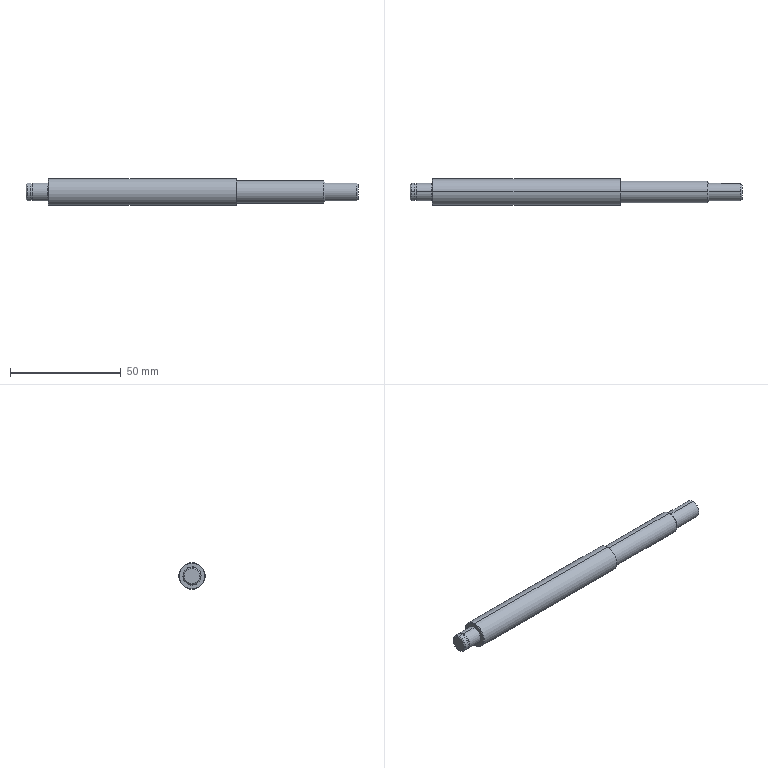Part | SolidWorks | features BaseBody 1 | 1 solid | 36 faces | box 150 x 12 x 12 mm | volume 13946 mm3 | cylinder 13 | plane 10 | cone 9 | spline 4 | commonest cylinder face diameters 8 x6 7.6 x2 10 x2 12 x2 3 x1
STEP:
#1=CARTESIAN_POINT('',(95.,0.,-5.1));
#2=VERTEX_POINT('',#1);
#3=CARTESIAN_POINT('',(95.,0.,5.1));
#4=VERTEX_POINT('',#3);
#5=CARTESIAN_POINT('',(95.,0.,-5.1));
#6=CARTESIAN_POINT('',(95.,10.2,-5.1));
#7=CARTESIAN_POINT('',(95.,10.2,5.1));
#8=CARTESIAN_POINT('',(95.,0.,5.1));
#9=(BOUNDED_CURVE()B_SPLINE_CURVE(3,(#5,#6,#7,#8),.UNSPECIFIED.,.F.,.F.)B_SPLINE_CURVE_WITH_KNOTS((4,4),(0.,0.5),.UNSPECIFIED.)CURVE()GEOMETRIC_REPRESENTATION_ITEM()RATIONAL_B_SPLINE_CURVE((1.,0.3333,0.3333,1.))REPRESENTATION_ITEM(''));
#10=EDGE_CURVE('',#2,#4,#9,.T.);
#11=ORIENTED_EDGE('',*,*,#10,.T.);
#12=CARTESIAN_POINT('',(95.1,0.,5.));
#13=VERTEX_POINT('',#12);
#14=CARTESIAN_POINT('',(95.1,0.,5.1));
#15=DIRECTION('',(0.,-1.,0.));
#16=DIRECTION('',(0.,0.,1.));
#17=AXIS2_PLACEMENT_3D('',#14,#15,#16);
#18=CIRCLE('',#17,0.1);
#19=EDGE_CURVE('',#4,#13,#18,.T.);
#20=ORIENTED_EDGE('',*,*,#19,.T.);
#21=CARTESIAN_POINT('',(95.1,0.,-5.));
#22=VERTEX_POINT('',#21);
#23=CARTESIAN_POINT('',(95.1,0.,0.));
#24=DIRECTION('',(1.,0.,0.));
#25=DIRECTION('',(0.,0.,-1.));
#26=AXIS2_PLACEMENT_3D('',#23,#24,#25);
#27=CIRCLE('',#26,5.);
#28=EDGE_CURVE('',#22,#13,#27,.T.);
#29=ORIENTED_EDGE('',*,*,#28,.F.);
#30=CARTESIAN_POINT('',(95.1,0.,-5.1));
#31=DIRECTION('',(0.,1.,0.));
#32=DIRECTION('',(0.,0.,-1.));
#33=AXIS2_PLACEMENT_3D('',#30,#31,#32);
#34=CIRCLE('',#33,0.1);
#35=EDGE_CURVE('',#2,#22,#34,.T.);
#36=ORIENTED_EDGE('',*,*,#35,.F.);
#37=EDGE_LOOP('',(#11,#20,#29,#36));
#38=FACE_OUTER_BOUND('',#37,.T.);
#39=CARTESIAN_POINT('',(95.,0.,-5.1));
#40=CARTESIAN_POINT('',(95.,10.2,-5.1));
#41=CARTESIAN_POINT('',(95.,10.2,5.1));
#42=CARTESIAN_POINT('',(95.,0.,5.1));
#43=CARTESIAN_POINT('',(95.,0.,-5.041));
#44=CARTESIAN_POINT('',(95.,10.083,-5.041));
#45=CARTESIAN_POINT('',(95.,10.083,5.041));
#46=CARTESIAN_POINT('',(95.,0.,5.041));
#47=CARTESIAN_POINT('',(95.041,0.,-5.));
#48=CARTESIAN_POINT('',(95.041,10.,-5.));
#49=CARTESIAN_POINT('',(95.041,10.,5.));
#50=CARTESIAN_POINT('',(95.041,0.,5.));
#51=CARTESIAN_POINT('',(95.1,0.,-5.));
#52=CARTESIAN_POINT('',(95.1,10.,-5.));
#53=CARTESIAN_POINT('',(95.1,10.,5.));
#54=CARTESIAN_POINT('',(95.1,0.,5.));
#55=(BOUNDED_SURFACE()B_SPLINE_SURFACE(3,3,((#39,#40,#41,#42),(#43,#44,#45,#46),(#47,#48,#49,#50),(#51,#52,#53,#54)),.UNSPECIFIED.,.F.,.F.,.T.)B_SPLINE_SURFACE_WITH_KNOTS((4,4),(4,4),(0.,1.),(0.,1.),.UNSPECIFIED.)GEOMETRIC_REPRESENTATION_ITEM()RATIONAL_B_SPLINE_SURFACE(((1.,0.3333,0.3333,1.),(0.8047,0.2682,0.2682,0.8047),(0.8047,0.2682,0.2682,0.8047),(1.,0.3333,0.3333,1.)))REPRESENTATION_ITEM('')SURFACE());
#56=ADVANCED_FACE('',(#38),#55,.F.);
#57=CARTESIAN_POINT('',(9.9,0.,4.));
#58=VERTEX_POINT('',#57);
#59=CARTESIAN_POINT('',(9.9,0.,-4.));
#60=VERTEX_POINT('',#59);
#61=CARTESIAN_POINT('',(9.9,0.,0.));
#62=DIRECTION('',(-1.,0.,0.));
#63=DIRECTION('',(0.,0.,-1.));
#64=AXIS2_PLACEMENT_3D('',#61,#62,#63);
#65=CIRCLE('',#64,4.);
#66=EDGE_CURVE('',#58,#60,#65,.T.);
#67=ORIENTED_EDGE('',*,*,#66,.F.);
#68=CARTESIAN_POINT('',(10.,0.,4.1));
#69=VERTEX_POINT('',#68);
#70=CARTESIAN_POINT('',(9.9,0.,4.1));
#71=DIRECTION('',(0.,-1.,0.));
#72=DIRECTION('',(0.,0.,1.));
#73=AXIS2_PLACEMENT_3D('',#70,#71,#72);
#74=CIRCLE('',#73,0.1);
#75=EDGE_CURVE('',#58,#69,#74,.T.);
#76=ORIENTED_EDGE('',*,*,#75,.T.);
#77=CARTESIAN_POINT('',(10.,0.,-4.1));
#78=VERTEX_POINT('',#77);
#79=CARTESIAN_POINT('',(10.,0.,4.1));
#80=CARTESIAN_POINT('',(10.,8.2,4.1));
#81=CARTESIAN_POINT('',(10.,8.2,-4.1));
#82=CARTESIAN_POINT('',(10.,0.,-4.1));
#83=(BOUNDED_CURVE()B_SPLINE_CURVE(3,(#79,#80,#81,#82),.UNSPECIFIED.,.F.,.F.)B_SPLINE_CURVE_WITH_KNOTS((4,4),(0.5,1.),.UNSPECIFIED.)CURVE()GEOMETRIC_REPRESENTATION_ITEM()RATIONAL_B_SPLINE_CURVE((1.,0.3333,0.3333,1.))REPRESENTATION_ITEM(''));
#84=EDGE_CURVE('',#69,#78,#83,.T.);
#85=ORIENTED_EDGE('',*,*,#84,.T.);
#86=CARTESIAN_POINT('',(9.9,0.,-4.1));
#87=DIRECTION('',(0.,1.,0.));
#88=DIRECTION('',(0.,0.,-1.));
#89=AXIS2_PLACEMENT_3D('',#86,#87,#88);
#90=CIRCLE('',#89,0.1);
#91=EDGE_CURVE('',#60,#78,#90,.T.);
#92=ORIENTED_EDGE('',*,*,#91,.F.);
#93=EDGE_LOOP('',(#67,#76,#85,#92));
#94=FACE_OUTER_BOUND('',#93,.T.);
#95=CARTESIAN_POINT('',(9.9,0.,-4.));
#96=CARTESIAN_POINT('',(9.9,8.,-4.));
#97=CARTESIAN_POINT('',(9.9,8.,4.));
#98=CARTESIAN_POINT('',(9.9,0.,4.));
#99=CARTESIAN_POINT('',(9.959,0.,-4.));
#100=CARTESIAN_POINT('',(9.959,8.,-4.));
#101=CARTESIAN_POINT('',(9.959,8.,4.));
#102=CARTESIAN_POINT('',(9.959,0.,4.));
#103=CARTESIAN_POINT('',(10.,0.,-4.041));
#104=CARTESIAN_POINT('',(10.,8.083,-4.041));
#105=CARTESIAN_POINT('',(10.,8.083,4.041));
#106=CARTESIAN_POINT('',(10.,0.,4.041));
#107=CARTESIAN_POINT('',(10.,0.,-4.1));
#108=CARTESIAN_POINT('',(10.,8.2,-4.1));
#109=CARTESIAN_POINT('',(10.,8.2,4.1));
#110=CARTESIAN_POINT('',(10.,0.,4.1));
#111=(BOUNDED_SURFACE()B_SPLINE_SURFACE(3,3,((#95,#96,#97,#98),(#99,#100,#101,#102),(#103,#104,#105,#106),(#107,#108,#109,#110)),.UNSPECIFIED.,.F.,.F.,.F.)B_SPLINE_SURFACE_WITH_KNOTS((4,4),(4,4),(0.,1.),(0.,1.),.UNSPECIFIED.)GEOMETRIC_REPRESENTATION_ITEM()RATIONAL_B_SPLINE_SURFACE(((1.,0.3333,0.3333,1.),(0.8047,0.2682,0.2682,0.8047),(0.8047,0.2682,0.2682,0.8047),(1.,0.3333,0.3333,1.)))REPRESENTATION_ITEM('')SURFACE());
#112=ADVANCED_FACE('',(#94),#111,.F.);
#113=CARTESIAN_POINT('',(95.,0.,6.));
#114=VERTEX_POINT('',#113);
#115=CARTESIAN_POINT('',(95.,0.,-6.));
#116=VERTEX_POINT('',#115);
#117=CARTESIAN_POINT('',(95.,0.,0.));
#118=DIRECTION('',(-1.,0.,0.));
#119=DIRECTION('',(0.,0.,1.));
#120=AXIS2_PLACEMENT_3D('',#117,#118,#119);
#121=CIRCLE('',#120,6.);
#122=EDGE_CURVE('',#114,#116,#121,.T.);
#123=ORIENTED_EDGE('',*,*,#122,.T.);
#124=CARTESIAN_POINT('',(10.3,0.,-6.));
#125=VERTEX_POINT('',#124);
#126=CARTESIAN_POINT('',(150.,0.,-6.));
#127=DIRECTION('',(-1.,0.,0.));
#128=VECTOR('',#127,1000.);
#129=LINE('',#126,#128);
#130=EDGE_CURVE('',#116,#125,#129,.T.);
#131=ORIENTED_EDGE('',*,*,#130,.T.);
#132=CARTESIAN_POINT('',(10.3,0.,6.));
#133=VERTEX_POINT('',#132);
#134=CARTESIAN_POINT('',(10.3,0.,0.));
#135=DIRECTION('',(1.,0.,0.));
#136=DIRECTION('',(0.,0.,1.));
#137=AXIS2_PLACEMENT_3D('',#134,#135,#136);
#138=CIRCLE('',#137,6.);
#139=EDGE_CURVE('',#125,#133,#138,.T.);
#140=ORIENTED_EDGE('',*,*,#139,.T.);
#141=CARTESIAN_POINT('',(150.,0.,6.));
#142=DIRECTION('',(-1.,0.,0.));
#143=VECTOR('',#142,1000.);
#144=LINE('',#141,#143);
#145=EDGE_CURVE('',#114,#133,#144,.T.);
#146=ORIENTED_EDGE('',*,*,#145,.F.);
#147=EDGE_LOOP('',(#123,#131,#140,#146));
#148=FACE_OUTER_BOUND('',#147,.T.);
#149=CARTESIAN_POINT('',(150.,0.,0.));
#150=DIRECTION('',(-1.,0.,0.));
#151=DIRECTION('',(0.,0.,1.));
#152=AXIS2_PLACEMENT_3D('',#149,#150,#151);
#153=CYLINDRICAL_SURFACE('',#152,6.);
#154=ADVANCED_FACE('',(#148),#153,.T.);
#155=CARTESIAN_POINT('',(10.,0.,-5.7));
#156=VERTEX_POINT('',#155);
#157=CARTESIAN_POINT('',(10.,0.,5.7));
#158=VERTEX_POINT('',#157);
#159=CARTESIAN_POINT('',(10.,0.,0.));
#160=DIRECTION('',(1.,0.,0.));
#161=DIRECTION('',(0.,0.,-1.));
#162=AXIS2_PLACEMENT_3D('',#159,#160,#161);
#163=CIRCLE('',#162,5.7);
#164=EDGE_CURVE('',#156,#158,#163,.T.);
#165=ORIENTED_EDGE('',*,*,#164,.T.);
#166=CARTESIAN_POINT('',(10.3,0.,6.));
#167=DIRECTION('',(0.7071,0.,0.7071));
#168=VECTOR('',#167,1000.);
#169=LINE('',#166,#168);
#170=EDGE_CURVE('',#158,#133,#169,.T.);
#171=ORIENTED_EDGE('',*,*,#170,.T.);
#172=ORIENTED_EDGE('',*,*,#139,.F.);
#173=CARTESIAN_POINT('',(10.3,0.,-6.));
#174=DIRECTION('',(0.7071,0.,-0.7071));
#175=VECTOR('',#174,1000.);
#176=LINE('',#173,#175);
#177=EDGE_CURVE('',#156,#125,#176,.T.);
#178=ORIENTED_EDGE('',*,*,#177,.F.);
#179=EDGE_LOOP('',(#165,#171,#172,#178));
#180=FACE_OUTER_BOUND('',#179,.T.);
#181=CARTESIAN_POINT('',(10.3,0.,0.));
#182=DIRECTION('',(1.,0.,0.));
#183=DIRECTION('',(0.,0.,-1.));
#184=AXIS2_PLACEMENT_3D('',#181,#182,#183);
#185=CONICAL_SURFACE('',#184,6.,0.7854);
#186=ADVANCED_FACE('',(#180),#185,.T.);
#187=CARTESIAN_POINT('',(134.5,0.,5.));
#188=VERTEX_POINT('',#187);
#189=CARTESIAN_POINT('',(134.5,0.,-5.));
#190=VERTEX_POINT('',#189);
#191=CARTESIAN_POINT('',(134.5,0.,0.));
#192=DIRECTION('',(-1.,0.,0.));
#193=DIRECTION('',(0.,0.,1.));
#194=AXIS2_PLACEMENT_3D('',#191,#192,#193);
#195=CIRCLE('',#194,5.);
#196=EDGE_CURVE('',#188,#190,#195,.T.);
#197=ORIENTED_EDGE('',*,*,#196,.T.);
#198=CARTESIAN_POINT('',(150.,0.,-5.));
#199=DIRECTION('',(-1.,0.,0.));
#200=VECTOR('',#199,1000.);
#201=LINE('',#198,#200);
#202=EDGE_CURVE('',#190,#22,#201,.T.);
#203=ORIENTED_EDGE('',*,*,#202,.T.);
#204=ORIENTED_EDGE('',*,*,#28,.T.);
#205=CARTESIAN_POINT('',(150.,0.,5.));
#206=DIRECTION('',(-1.,0.,0.));
#207=VECTOR('',#206,1000.);
#208=LINE('',#205,#207);
#209=EDGE_CURVE('',#188,#13,#208,.T.);
#210=ORIENTED_EDGE('',*,*,#209,.F.);
#211=EDGE_LOOP('',(#197,#203,#204,#210));
#212=FACE_OUTER_BOUND('',#211,.T.);
#213=CARTESIAN_POINT('',(150.,0.,0.));
#214=DIRECTION('',(-1.,0.,0.));
#215=DIRECTION('',(0.,0.,1.));
#216=AXIS2_PLACEMENT_3D('',#213,#214,#215);
#217=CYLINDRICAL_SURFACE('',#216,5.);
#218=ADVANCED_FACE('',(#212),#217,.T.);
#219=ORIENTED_EDGE('',*,*,#66,.T.);
#220=CARTESIAN_POINT('',(3.,0.,-4.));
#221=VERTEX_POINT('',#220);
#222=CARTESIAN_POINT('',(150.,0.,-4.));
#223=DIRECTION('',(-1.,0.,0.));
#224=VECTOR('',#223,1000.);
#225=LINE('',#222,#224);
#226=EDGE_CURVE('',#60,#221,#225,.T.);
#227=ORIENTED_EDGE('',*,*,#226,.T.);
#228=CARTESIAN_POINT('',(3.,0.,4.));
#229=VERTEX_POINT('',#228);
#230=CARTESIAN_POINT('',(3.,0.,0.));
#231=DIRECTION('',(1.,0.,0.));
#232=DIRECTION('',(0.,0.,1.));
#233=AXIS2_PLACEMENT_3D('',#230,#231,#232);
#234=CIRCLE('',#233,4.);
#235=EDGE_CURVE('',#221,#229,#234,.T.);
#236=ORIENTED_EDGE('',*,*,#235,.T.);
#237=CARTESIAN_POINT('',(150.,0.,4.));
#238=DIRECTION('',(-1.,0.,0.));
#239=VECTOR('',#238,1000.);
#240=LINE('',#237,#239);
#241=EDGE_CURVE('',#58,#229,#240,.T.);
#242=ORIENTED_EDGE('',*,*,#241,.F.);
#243=EDGE_LOOP('',(#219,#227,#236,#242));
#244=FACE_OUTER_BOUND('',#243,.T.);
#245=CARTESIAN_POINT('',(150.,0.,0.));
#246=DIRECTION('',(-1.,0.,0.));
#247=DIRECTION('',(0.,0.,1.));
#248=AXIS2_PLACEMENT_3D('',#245,#246,#247);
#249=CYLINDRICAL_SURFACE('',#248,4.);
#250=ADVANCED_FACE('',(#244),#249,.T.);
#251=CARTESIAN_POINT('',(135.,0.,4.5));
#252=VERTEX_POINT('',#251);
#253=CARTESIAN_POINT('',(135.,0.,-4.5));
#254=VERTEX_POINT('',#253);
#255=CARTESIAN_POINT('',(135.,0.,0.));
#256=DIRECTION('',(-1.,0.,0.));
#257=DIRECTION('',(0.,0.,1.));
#258=AXIS2_PLACEMENT_3D('',#255,#256,#257);
#259=CIRCLE('',#258,4.5);
#260=EDGE_CURVE('',#252,#254,#259,.T.);
#261=ORIENTED_EDGE('',*,*,#260,.T.);
#262=CARTESIAN_POINT('',(134.5,0.,-5.));
#263=DIRECTION('',(-0.7071,0.,-0.7071));
#264=VECTOR('',#263,1000.);
#265=LINE('',#262,#264);
#266=EDGE_CURVE('',#254,#190,#265,.T.);
#267=ORIENTED_EDGE('',*,*,#266,.T.);
#268=ORIENTED_EDGE('',*,*,#196,.F.);
#269=CARTESIAN_POINT('',(134.5,0.,5.));
#270=DIRECTION('',(-0.7071,0.,0.7071));
#271=VECTOR('',#270,1000.);
#272=LINE('',#269,#271);
#273=EDGE_CURVE('',#252,#188,#272,.T.);
#274=ORIENTED_EDGE('',*,*,#273,.F.);
#275=EDGE_LOOP('',(#261,#267,#268,#274));
#276=FACE_OUTER_BOUND('',#275,.T.);
#277=CARTESIAN_POINT('',(134.5,0.,0.));
#278=DIRECTION('',(-1.,0.,0.));
#279=DIRECTION('',(0.,0.,1.));
#280=AXIS2_PLACEMENT_3D('',#277,#278,#279);
#281=CONICAL_SURFACE('',#280,5.,0.7854);
#282=ADVANCED_FACE('',(#276),#281,.T.);
#283=CARTESIAN_POINT('',(3.,0.,3.8));
#284=VERTEX_POINT('',#283);
#285=CARTESIAN_POINT('',(3.,0.,-3.8));
#286=VERTEX_POINT('',#285);
#287=CARTESIAN_POINT('',(3.,0.,0.));
#288=DIRECTION('',(-1.,0.,0.));
#289=DIRECTION('',(0.,0.,1.));
#290=AXIS2_PLACEMENT_3D('',#287,#288,#289);
#291=CIRCLE('',#290,3.8);
#292=EDGE_CURVE('',#284,#286,#291,.T.);
#293=ORIENTED_EDGE('',*,*,#292,.T.);
#294=CARTESIAN_POINT('',(2.1,0.,-3.8));
#295=VERTEX_POINT('',#294);
#296=CARTESIAN_POINT('',(150.,0.,-3.8));
#297=DIRECTION('',(-1.,0.,0.));
#298=VECTOR('',#297,1000.);
#299=LINE('',#296,#298);
#300=EDGE_CURVE('',#286,#295,#299,.T.);
#301=ORIENTED_EDGE('',*,*,#300,.T.);
#302=CARTESIAN_POINT('',(2.1,0.,3.8));
#303=VERTEX_POINT('',#302);
#304=CARTESIAN_POINT('',(2.1,0.,0.));
#305=DIRECTION('',(1.,0.,0.));
#306=DIRECTION('',(0.,0.,1.));
#307=AXIS2_PLACEMENT_3D('',#304,#305,#306);
#308=CIRCLE('',#307,3.8);
#309=EDGE_CURVE('',#295,#303,#308,.T.);
#310=ORIENTED_EDGE('',*,*,#309,.T.);
#311=CARTESIAN_POINT('',(150.,0.,3.8));
#312=DIRECTION('',(-1.,0.,0.));
#313=VECTOR('',#312,1000.);
#314=LINE('',#311,#313);
#315=EDGE_CURVE('',#284,#303,#314,.T.);
#316=ORIENTED_EDGE('',*,*,#315,.F.);
#317=EDGE_LOOP('',(#293,#301,#310,#316));
#318=FACE_OUTER_BOUND('',#317,.T.);
#319=CARTESIAN_POINT('',(150.,0.,0.));
#320=DIRECTION('',(-1.,0.,0.));
#321=DIRECTION('',(0.,0.,1.));
#322=AXIS2_PLACEMENT_3D('',#319,#320,#321);
#323=CYLINDRICAL_SURFACE('',#322,3.8);
#324=ADVANCED_FACE('',(#318),#323,.T.);
#325=CARTESIAN_POINT('',(149.5,3.708,-1.5));
#326=VERTEX_POINT('',#325);
#327=CARTESIAN_POINT('',(149.5,0.,-4.));
#328=VERTEX_POINT('',#327);
#329=CARTESIAN_POINT('',(149.5,0.,0.));
#330=DIRECTION('',(-1.,0.,0.));
#331=DIRECTION('',(0.,0.,1.));
#332=AXIS2_PLACEMENT_3D('',#329,#330,#331);
#333=CIRCLE('',#332,4.);
#334=EDGE_CURVE('',#326,#328,#333,.T.);
#335=ORIENTED_EDGE('',*,*,#334,.T.);
#336=CARTESIAN_POINT('',(135.,0.,-4.));
#337=VERTEX_POINT('',#336);
#338=CARTESIAN_POINT('',(150.,0.,-4.));
#339=DIRECTION('',(-1.,0.,0.));
#340=VECTOR('',#339,1000.);
#341=LINE('',#338,#340);
#342=EDGE_CURVE('',#328,#337,#341,.T.);
#343=ORIENTED_EDGE('',*,*,#342,.T.);
#344=CARTESIAN_POINT('',(135.,0.,4.));
#345=VERTEX_POINT('',#344);
#346=CARTESIAN_POINT('',(135.,0.,0.));
#347=DIRECTION('',(1.,0.,0.));
#348=DIRECTION('',(0.,0.,1.));
#349=AXIS2_PLACEMENT_3D('',#346,#347,#348);
#350=CIRCLE('',#349,4.);
#351=EDGE_CURVE('',#337,#345,#350,.T.);
#352=ORIENTED_EDGE('',*,*,#351,.T.);
#353=CARTESIAN_POINT('',(149.5,0.,4.));
#354=VERTEX_POINT('',#353);
#355=CARTESIAN_POINT('',(150.,0.,4.));
#356=DIRECTION('',(-1.,0.,0.));
#357=VECTOR('',#356,1000.);
#358=LINE('',#355,#357);
#359=EDGE_CURVE('',#354,#345,#358,.T.);
#360=ORIENTED_EDGE('',*,*,#359,.F.);
#361=CARTESIAN_POINT('',(149.5,3.708,1.5));
#362=VERTEX_POINT('',#361);
#363=CARTESIAN_POINT('',(149.5,0.,0.));
#364=DIRECTION('',(-1.,0.,0.));
#365=DIRECTION('',(0.,0.,1.));
#366=AXIS2_PLACEMENT_3D('',#363,#364,#365);
#367=CIRCLE('',#366,4.);
#368=EDGE_CURVE('',#354,#362,#367,.T.);
#369=ORIENTED_EDGE('',*,*,#368,.T.);
#370=CARTESIAN_POINT('',(141.5,3.708,1.5));
#371=VERTEX_POINT('',#370);
#372=CARTESIAN_POINT('',(150.,3.708,1.5));
#373=DIRECTION('',(-1.,0.,0.));
#374=VECTOR('',#373,1000.);
#375=LINE('',#372,#374);
#376=EDGE_CURVE('',#362,#371,#375,.T.);
#377=ORIENTED_EDGE('',*,*,#376,.T.);
#378=CARTESIAN_POINT('',(141.5,3.708,-1.5));
#379=VERTEX_POINT('',#378);
#380=CARTESIAN_POINT('',(141.5,3.708,1.5));
#381=CARTESIAN_POINT('',(141.4,3.708,1.5));
#382=CARTESIAN_POINT('',(141.302,3.712,1.49));
#383=CARTESIAN_POINT('',(141.109,3.727,1.451));
#384=CARTESIAN_POINT('',(141.013,3.739,1.422));
#385=CARTESIAN_POINT('',(140.742,3.781,1.309));
#386=CARTESIAN_POINT('',(140.577,3.819,1.198));
#387=CARTESIAN_POINT('',(140.303,3.894,0.924));
#388=CARTESIAN_POINT('',(140.191,3.932,0.7582));
#389=CARTESIAN_POINT('',(140.078,3.971,0.488));
#390=CARTESIAN_POINT('',(140.049,3.982,0.3926));
#391=CARTESIAN_POINT('',(140.01,3.996,0.1986));
#392=CARTESIAN_POINT('',(140.,4.,0.1006));
#393=CARTESIAN_POINT('',(140.,4.,-0.09712));
#394=CARTESIAN_POINT('',(140.01,3.996,-0.1975));
#395=CARTESIAN_POINT('',(140.048,3.982,-0.3907));
#396=CARTESIAN_POINT('',(140.077,3.972,-0.4847));
#397=CARTESIAN_POINT('',(140.191,3.932,-0.759));
#398=CARTESIAN_POINT('',(140.302,3.895,-0.9229));
#399=CARTESIAN_POINT('',(140.508,3.838,-1.129));
#400=CARTESIAN_POINT('',(140.583,3.819,-1.191));
#401=CARTESIAN_POINT('',(140.744,3.783,-1.299));
#402=CARTESIAN_POINT('',(140.832,3.767,-1.347));
#403=CARTESIAN_POINT('',(141.102,3.725,-1.459));
#404=CARTESIAN_POINT('',(141.3,3.708,-1.5));
#405=CARTESIAN_POINT('',(141.5,3.708,-1.5));
#406=B_SPLINE_CURVE_WITH_KNOTS('',3,(#380,#381,#382,#383,#384,#385,#386,#387,#388,#389,#390,#391,#392,#393,#394,#395,#396,#397,#398,#399,#400,#401,#402,#403,#404,#405),.UNSPECIFIED.,.F.,.F.,(4,2,2,2,2,2,2,2,2,2,2,2,4),(0.,0.0002957,0.0005914,0.001183,0.001774,0.00207,0.002366,0.002661,0.002957,0.003548,0.003844,0.00414,0.004731),.UNSPECIFIED.);
#407=EDGE_CURVE('',#371,#379,#406,.T.);
#408=ORIENTED_EDGE('',*,*,#407,.T.);
#409=CARTESIAN_POINT('',(150.,3.708,-1.5));
#410=DIRECTION('',(1.,0.,0.));
#411=VECTOR('',#410,1000.);
#412=LINE('',#409,#411);
#413=EDGE_CURVE('',#379,#326,#412,.T.);
#414=ORIENTED_EDGE('',*,*,#413,.T.);
#415=EDGE_LOOP('',(#335,#343,#352,#360,#369,#377,#408,#414));
#416=FACE_OUTER_BOUND('',#415,.T.);
#417=CARTESIAN_POINT('',(150.,0.,0.));
#418=DIRECTION('',(-1.,0.,0.));
#419=DIRECTION('',(0.,0.,1.));
#420=AXIS2_PLACEMENT_3D('',#417,#418,#419);
#421=CYLINDRICAL_SURFACE('',#420,4.);
#422=ADVANCED_FACE('',(#416),#421,.T.);
#423=CARTESIAN_POINT('',(150.,3.162,-1.5));
#424=VERTEX_POINT('',#423);
#425=CARTESIAN_POINT('',(150.,0.,-3.5));
#426=VERTEX_POINT('',#425);
#427=CARTESIAN_POINT('',(150.,0.,0.));
#428=DIRECTION('',(-1.,0.,0.));
#429=DIRECTION('',(0.,0.,1.));
#430=AXIS2_PLACEMENT_3D('',#427,#428,#429);
#431=CIRCLE('',#430,3.5);
#432=EDGE_CURVE('',#424,#426,#431,.T.);
#433=ORIENTED_EDGE('',*,*,#432,.T.);
#434=CARTESIAN_POINT('',(149.5,0.,-4.));
#435=DIRECTION('',(-0.7071,0.,-0.7071));
#436=VECTOR('',#435,1000.);
#437=LINE('',#434,#436);
#438=EDGE_CURVE('',#426,#328,#437,.T.);
#439=ORIENTED_EDGE('',*,*,#438,.T.);
#440=ORIENTED_EDGE('',*,*,#334,.F.);
#441=CARTESIAN_POINT('',(149.5,3.708,-1.5));
#442=CARTESIAN_POINT('',(149.668,3.527,-1.5));
#443=CARTESIAN_POINT('',(149.835,3.345,-1.5));
#444=CARTESIAN_POINT('',(150.,3.162,-1.5));
#445=B_SPLINE_CURVE_WITH_KNOTS('',3,(#441,#442,#443,#444),.UNSPECIFIED.,.F.,.F.,(4,4),(0.,0.0007402),.UNSPECIFIED.);
#446=EDGE_CURVE('',#326,#424,#445,.T.);
#447=ORIENTED_EDGE('',*,*,#446,.T.);
#448=EDGE_LOOP('',(#433,#439,#440,#447));
#449=FACE_OUTER_BOUND('',#448,.T.);
#450=CARTESIAN_POINT('',(149.5,0.,0.));
#451=DIRECTION('',(-1.,0.,0.));
#452=DIRECTION('',(0.,0.,1.));
#453=AXIS2_PLACEMENT_3D('',#450,#451,#452);
#454=CONICAL_SURFACE('',#453,4.,0.7854);
#455=ADVANCED_FACE('',(#449),#454,.T.);
#456=ORIENTED_EDGE('',*,*,#438,.F.);
#457=CARTESIAN_POINT('',(150.,0.,3.5));
#458=VERTEX_POINT('',#457);
#459=CARTESIAN_POINT('',(150.,0.,0.));
#460=DIRECTION('',(-1.,0.,0.));
#461=DIRECTION('',(0.,0.,1.));
#462=AXIS2_PLACEMENT_3D('',#459,#460,#461);
#463=CIRCLE('',#462,3.5);
#464=EDGE_CURVE('',#426,#458,#463,.T.);
#465=ORIENTED_EDGE('',*,*,#464,.T.);
#466=CARTESIAN_POINT('',(149.5,0.,4.));
#467=DIRECTION('',(-0.7071,0.,0.7071));
#468=VECTOR('',#467,1000.);
#469=LINE('',#466,#468);
#470=EDGE_CURVE('',#458,#354,#469,.T.);
#471=ORIENTED_EDGE('',*,*,#470,.T.);
#472=CARTESIAN_POINT('',(149.5,0.,0.));
#473=DIRECTION('',(-1.,0.,0.));
#474=DIRECTION('',(0.,0.,1.));
#475=AXIS2_PLACEMENT_3D('',#472,#473,#474);
#476=CIRCLE('',#475,4.);
#477=EDGE_CURVE('',#328,#354,#476,.T.);
#478=ORIENTED_EDGE('',*,*,#477,.F.);
#479=EDGE_LOOP('',(#456,#465,#471,#478));
#480=FACE_OUTER_BOUND('',#479,.T.);
#481=CARTESIAN_POINT('',(149.5,0.,0.));
#482=DIRECTION('',(-1.,0.,0.));
#483=DIRECTION('',(0.,0.,1.));
#484=AXIS2_PLACEMENT_3D('',#481,#482,#483);
#485=CONICAL_SURFACE('',#484,4.,0.7854);
#486=ADVANCED_FACE('',(#480),#485,.T.);
#487=CARTESIAN_POINT('',(2.1,0.,4.));
#488=VERTEX_POINT('',#487);
#489=CARTESIAN_POINT('',(2.1,0.,-4.));
#490=VERTEX_POINT('',#489);
#491=CARTESIAN_POINT('',(2.1,0.,0.));
#492=DIRECTION('',(-1.,0.,0.));
#493=DIRECTION('',(0.,0.,1.));
#494=AXIS2_PLACEMENT_3D('',#491,#492,#493);
#495=CIRCLE('',#494,4.);
#496=EDGE_CURVE('',#488,#490,#495,.T.);
#497=ORIENTED_EDGE('',*,*,#496,.T.);
#498=CARTESIAN_POINT('',(0.5,0.,-4.));
#499=VERTEX_POINT('',#498);
#500=CARTESIAN_POINT('',(150.,0.,-4.));
#501=DIRECTION('',(-1.,0.,0.));
#502=VECTOR('',#501,1000.);
#503=LINE('',#500,#502);
#504=EDGE_CURVE('',#490,#499,#503,.T.);
#505=ORIENTED_EDGE('',*,*,#504,.T.);
#506=CARTESIAN_POINT('',(0.5,0.,4.));
#507=VERTEX_POINT('',#506);
#508=CARTESIAN_POINT('',(0.5,0.,0.));
#509=DIRECTION('',(1.,0.,0.));
#510=DIRECTION('',(0.,0.,1.));
#511=AXIS2_PLACEMENT_3D('',#508,#509,#510);
#512=CIRCLE('',#511,4.);
#513=EDGE_CURVE('',#499,#507,#512,.T.);
#514=ORIENTED_EDGE('',*,*,#513,.T.);
#515=CARTESIAN_POINT('',(150.,0.,4.));
#516=DIRECTION('',(-1.,0.,0.));
#517=VECTOR('',#516,1000.);
#518=LINE('',#515,#517);
#519=EDGE_CURVE('',#488,#507,#518,.T.);
#520=ORIENTED_EDGE('',*,*,#519,.F.);
#521=EDGE_LOOP('',(#497,#505,#514,#520));
#522=FACE_OUTER_BOUND('',#521,.T.);
#523=CARTESIAN_POINT('',(150.,0.,0.));
#524=DIRECTION('',(-1.,0.,0.));
#525=DIRECTION('',(0.,0.,1.));
#526=AXIS2_PLACEMENT_3D('',#523,#524,#525);
#527=CYLINDRICAL_SURFACE('',#526,4.);
#528=ADVANCED_FACE('',(#522),#527,.T.);
#529=CARTESIAN_POINT('',(0.,0.,-3.5));
#530=VERTEX_POINT('',#529);
#531=CARTESIAN_POINT('',(0.,0.,3.5));
#532=VERTEX_POINT('',#531);
#533=CARTESIAN_POINT('',(0.,0.,0.));
#534=DIRECTION('',(1.,0.,0.));
#535=DIRECTION('',(0.,0.,-1.));
#536=AXIS2_PLACEMENT_3D('',#533,#534,#535);
#537=CIRCLE('',#536,3.5);
#538=EDGE_CURVE('',#530,#532,#537,.T.);
#539=ORIENTED_EDGE('',*,*,#538,.T.);
#540=CARTESIAN_POINT('',(0.5,0.,4.));
#541=DIRECTION('',(0.7071,0.,0.7071));
#542=VECTOR('',#541,1000.);
#543=LINE('',#540,#542);
#544=EDGE_CURVE('',#532,#507,#543,.T.);
#545=ORIENTED_EDGE('',*,*,#544,.T.);
#546=ORIENTED_EDGE('',*,*,#513,.F.);
#547=CARTESIAN_POINT('',(0.5,0.,-4.));
#548=DIRECTION('',(0.7071,0.,-0.7071));
#549=VECTOR('',#548,1000.);
#550=LINE('',#547,#549);
#551=EDGE_CURVE('',#530,#499,#550,.T.);
#552=ORIENTED_EDGE('',*,*,#551,.F.);
#553=EDGE_LOOP('',(#539,#545,#546,#552));
#554=FACE_OUTER_BOUND('',#553,.T.);
#555=CARTESIAN_POINT('',(0.5,0.,0.));
#556=DIRECTION('',(1.,0.,0.));
#557=DIRECTION('',(0.,0.,-1.));
#558=AXIS2_PLACEMENT_3D('',#555,#556,#557);
#559=CONICAL_SURFACE('',#558,4.,0.7854);
#560=ADVANCED_FACE('',(#554),#559,.T.);
#561=ORIENTED_EDGE('',*,*,#130,.F.);
#562=CARTESIAN_POINT('',(95.,0.,0.));
#563=DIRECTION('',(-1.,0.,0.));
#564=DIRECTION('',(0.,0.,1.));
#565=AXIS2_PLACEMENT_3D('',#562,#563,#564);
#566=CIRCLE('',#565,6.);
#567=EDGE_CURVE('',#116,#114,#566,.T.);
#568=ORIENTED_EDGE('',*,*,#567,.T.);
#569=ORIENTED_EDGE('',*,*,#145,.T.);
#570=CARTESIAN_POINT('',(10.3,0.,0.));
#571=DIRECTION('',(1.,0.,0.));
#572=DIRECTION('',(0.,0.,1.));
#573=AXIS2_PLACEMENT_3D('',#570,#571,#572);
#574=CIRCLE('',#573,6.);
#575=EDGE_CURVE('',#133,#125,#574,.T.);
#576=ORIENTED_EDGE('',*,*,#575,.T.);
#577=EDGE_LOOP('',(#561,#568,#569,#576));
#578=FACE_OUTER_BOUND('',#577,.T.);
#579=CARTESIAN_POINT('',(150.,0.,0.));
#580=DIRECTION('',(-1.,0.,0.));
#581=DIRECTION('',(0.,0.,1.));
#582=AXIS2_PLACEMENT_3D('',#579,#580,#581);
#583=CYLINDRICAL_SURFACE('',#582,6.);
#584=ADVANCED_FACE('',(#578),#583,.T.);
#585=ORIENTED_EDGE('',*,*,#170,.F.);
#586=CARTESIAN_POINT('',(10.,0.,0.));
#587=DIRECTION('',(1.,0.,0.));
#588=DIRECTION('',(0.,0.,-1.));
#589=AXIS2_PLACEMENT_3D('',#586,#587,#588);
#590=CIRCLE('',#589,5.7);
#591=EDGE_CURVE('',#158,#156,#590,.T.);
#592=ORIENTED_EDGE('',*,*,#591,.T.);
#593=ORIENTED_EDGE('',*,*,#177,.T.);
#594=ORIENTED_EDGE('',*,*,#575,.F.);
#595=EDGE_LOOP('',(#585,#592,#593,#594));
#596=FACE_OUTER_BOUND('',#595,.T.);
#597=CARTESIAN_POINT('',(10.3,0.,0.));
#598=DIRECTION('',(1.,0.,0.));
#599=DIRECTION('',(0.,0.,-1.));
#600=AXIS2_PLACEMENT_3D('',#597,#598,#599);
#601=CONICAL_SURFACE('',#600,6.,0.7854);
#602=ADVANCED_FACE('',(#596),#601,.T.);
#603=ORIENTED_EDGE('',*,*,#122,.F.);
#604=ORIENTED_EDGE('',*,*,#567,.F.);
#605=EDGE_LOOP('',(#603,#604));
#606=FACE_OUTER_BOUND('',#605,.T.);
#607=ORIENTED_EDGE('',*,*,#10,.F.);
#608=CARTESIAN_POINT('',(95.,0.,5.1));
#609=CARTESIAN_POINT('',(95.,-10.2,5.1));
#610=CARTESIAN_POINT('',(95.,-10.2,-5.1));
#611=CARTESIAN_POINT('',(95.,0.,-5.1));
#612=(BOUNDED_CURVE()B_SPLINE_CURVE(3,(#608,#609,#610,#611),.UNSPECIFIED.,.F.,.F.)B_SPLINE_CURVE_WITH_KNOTS((4,4),(0.5,1.),.UNSPECIFIED.)CURVE()GEOMETRIC_REPRESENTATION_ITEM()RATIONAL_B_SPLINE_CURVE((1.,0.3333,0.3333,1.))REPRESENTATION_ITEM(''));
#613=EDGE_CURVE('',#4,#2,#612,.T.);
#614=ORIENTED_EDGE('',*,*,#613,.F.);
#615=EDGE_LOOP('',(#607,#614));
#616=FACE_BOUND('',#615,.T.);
#617=CARTESIAN_POINT('',(95.,6.,0.));
#618=DIRECTION('',(-1.,0.,0.));
#619=DIRECTION('',(0.,0.,1.));
#620=AXIS2_PLACEMENT_3D('',#617,#618,#619);
#621=PLANE('',#620);
#622=ADVANCED_FACE('',(#606,#616),#621,.F.);
#623=CARTESIAN_POINT('',(10.,0.,-4.1));
#624=CARTESIAN_POINT('',(10.,-8.2,-4.1));
#625=CARTESIAN_POINT('',(10.,-8.2,4.1));
#626=CARTESIAN_POINT('',(10.,0.,4.1));
#627=(BOUNDED_CURVE()B_SPLINE_CURVE(3,(#623,#624,#625,#626),.UNSPECIFIED.,.F.,.F.)B_SPLINE_CURVE_WITH_KNOTS((4,4),(0.,0.5),.UNSPECIFIED.)CURVE()GEOMETRIC_REPRESENTATION_ITEM()RATIONAL_B_SPLINE_CURVE((1.,0.3333,0.3333,1.))REPRESENTATION_ITEM(''));
#628=EDGE_CURVE('',#78,#69,#627,.T.);
#629=ORIENTED_EDGE('',*,*,#628,.F.);
#630=ORIENTED_EDGE('',*,*,#84,.F.);
#631=EDGE_LOOP('',(#629,#630));
#632=FACE_BOUND('',#631,.T.);
#633=ORIENTED_EDGE('',*,*,#164,.F.);
#634=ORIENTED_EDGE('',*,*,#591,.F.);
#635=EDGE_LOOP('',(#633,#634));
#636=FACE_OUTER_BOUND('',#635,.T.);
#637=CARTESIAN_POINT('',(10.,4.1,0.));
#638=DIRECTION('',(1.,0.,0.));
#639=DIRECTION('',(0.,0.,-1.));
#640=AXIS2_PLACEMENT_3D('',#637,#638,#639);
#641=PLANE('',#640);
#642=ADVANCED_FACE('',(#632,#636),#641,.F.);
#643=ORIENTED_EDGE('',*,*,#19,.F.);
#644=ORIENTED_EDGE('',*,*,#613,.T.);
#645=ORIENTED_EDGE('',*,*,#35,.T.);
#646=CARTESIAN_POINT('',(95.1,0.,0.));
#647=DIRECTION('',(1.,0.,0.));
#648=DIRECTION('',(0.,0.,-1.));
#649=AXIS2_PLACEMENT_3D('',#646,#647,#648);
#650=CIRCLE('',#649,5.);
#651=EDGE_CURVE('',#13,#22,#650,.T.);
#652=ORIENTED_EDGE('',*,*,#651,.F.);
#653=EDGE_LOOP('',(#643,#644,#645,#652));
#654=FACE_OUTER_BOUND('',#653,.T.);
#655=CARTESIAN_POINT('',(95.,0.,5.1));
#656=CARTESIAN_POINT('',(95.,-10.2,5.1));
#657=CARTESIAN_POINT('',(95.,-10.2,-5.1));
#658=CARTESIAN_POINT('',(95.,0.,-5.1));
#659=CARTESIAN_POINT('',(95.,0.,5.041));
#660=CARTESIAN_POINT('',(95.,-10.083,5.041));
#661=CARTESIAN_POINT('',(95.,-10.083,-5.041));
#662=CARTESIAN_POINT('',(95.,0.,-5.041));
#663=CARTESIAN_POINT('',(95.041,0.,5.));
#664=CARTESIAN_POINT('',(95.041,-10.,5.));
#665=CARTESIAN_POINT('',(95.041,-10.,-5.));
#666=CARTESIAN_POINT('',(95.041,0.,-5.));
#667=CARTESIAN_POINT('',(95.1,0.,5.));
#668=CARTESIAN_POINT('',(95.1,-10.,5.));
#669=CARTESIAN_POINT('',(95.1,-10.,-5.));
#670=CARTESIAN_POINT('',(95.1,0.,-5.));
#671=(BOUNDED_SURFACE()B_SPLINE_SURFACE(3,3,((#655,#656,#657,#658),(#659,#660,#661,#662),(#663,#664,#665,#666),(#667,#668,#669,#670)),.UNSPECIFIED.,.F.,.F.,.F.)B_SPLINE_SURFACE_WITH_KNOTS((4,4),(4,4),(0.,1.),(0.,1.),.UNSPECIFIED.)GEOMETRIC_REPRESENTATION_ITEM()RATIONAL_B_SPLINE_SURFACE(((1.,0.3333,0.3333,1.),(0.8047,0.2682,0.2682,0.8047),(0.8047,0.2682,0.2682,0.8047),(1.,0.3333,0.3333,1.)))REPRESENTATION_ITEM('')SURFACE());
#672=ADVANCED_FACE('',(#654),#671,.F.);
#673=ORIENTED_EDGE('',*,*,#75,.F.);
#674=CARTESIAN_POINT('',(9.9,0.,0.));
#675=DIRECTION('',(-1.,0.,0.));
#676=DIRECTION('',(0.,0.,-1.));
#677=AXIS2_PLACEMENT_3D('',#674,#675,#676);
#678=CIRCLE('',#677,4.);
#679=EDGE_CURVE('',#60,#58,#678,.T.);
#680=ORIENTED_EDGE('',*,*,#679,.F.);
#681=ORIENTED_EDGE('',*,*,#91,.T.);
#682=ORIENTED_EDGE('',*,*,#628,.T.);
#683=EDGE_LOOP('',(#673,#680,#681,#682));
#684=FACE_OUTER_BOUND('',#683,.T.);
#685=CARTESIAN_POINT('',(9.9,0.,4.));
#686=CARTESIAN_POINT('',(9.9,-8.,4.));
#687=CARTESIAN_POINT('',(9.9,-8.,-4.));
#688=CARTESIAN_POINT('',(9.9,0.,-4.));
#689=CARTESIAN_POINT('',(9.959,0.,4.));
#690=CARTESIAN_POINT('',(9.959,-8.,4.));
#691=CARTESIAN_POINT('',(9.959,-8.,-4.));
#692=CARTESIAN_POINT('',(9.959,0.,-4.));
#693=CARTESIAN_POINT('',(10.,0.,4.041));
#694=CARTESIAN_POINT('',(10.,-8.083,4.041));
#695=CARTESIAN_POINT('',(10.,-8.083,-4.041));
#696=CARTESIAN_POINT('',(10.,0.,-4.041));
#697=CARTESIAN_POINT('',(10.,0.,4.1));
#698=CARTESIAN_POINT('',(10.,-8.2,4.1));
#699=CARTESIAN_POINT('',(10.,-8.2,-4.1));
#700=CARTESIAN_POINT('',(10.,0.,-4.1));
#701=(BOUNDED_SURFACE()B_SPLINE_SURFACE(3,3,((#685,#686,#687,#688),(#689,#690,#691,#692),(#693,#694,#695,#696),(#697,#698,#699,#700)),.UNSPECIFIED.,.F.,.F.,.T.)B_SPLINE_SURFACE_WITH_KNOTS((4,4),(4,4),(0.,1.),(0.,1.),.UNSPECIFIED.)GEOMETRIC_REPRESENTATION_ITEM()RATIONAL_B_SPLINE_SURFACE(((1.,0.3333,0.3333,1.),(0.8047,0.2682,0.2682,0.8047),(0.8047,0.2682,0.2682,0.8047),(1.,0.3333,0.3333,1.)))REPRESENTATION_ITEM('')SURFACE());
#702=ADVANCED_FACE('',(#684),#701,.F.);
#703=ORIENTED_EDGE('',*,*,#202,.F.);
#704=CARTESIAN_POINT('',(134.5,0.,0.));
#705=DIRECTION('',(-1.,0.,0.));
#706=DIRECTION('',(0.,0.,1.));
#707=AXIS2_PLACEMENT_3D('',#704,#705,#706);
#708=CIRCLE('',#707,5.);
#709=EDGE_CURVE('',#190,#188,#708,.T.);
#710=ORIENTED_EDGE('',*,*,#709,.T.);
#711=ORIENTED_EDGE('',*,*,#209,.T.);
#712=ORIENTED_EDGE('',*,*,#651,.T.);
#713=EDGE_LOOP('',(#703,#710,#711,#712));
#714=FACE_OUTER_BOUND('',#713,.T.);
#715=CARTESIAN_POINT('',(150.,0.,0.));
#716=DIRECTION('',(-1.,0.,0.));
#717=DIRECTION('',(0.,0.,1.));
#718=AXIS2_PLACEMENT_3D('',#715,#716,#717);
#719=CYLINDRICAL_SURFACE('',#718,5.);
#720=ADVANCED_FACE('',(#714),#719,.T.);
#721=ORIENTED_EDGE('',*,*,#226,.F.);
#722=ORIENTED_EDGE('',*,*,#679,.T.);
#723=ORIENTED_EDGE('',*,*,#241,.T.);
#724=CARTESIAN_POINT('',(3.,0.,0.));
#725=DIRECTION('',(1.,0.,0.));
#726=DIRECTION('',(0.,0.,1.));
#727=AXIS2_PLACEMENT_3D('',#724,#725,#726);
#728=CIRCLE('',#727,4.);
#729=EDGE_CURVE('',#229,#221,#728,.T.);
#730=ORIENTED_EDGE('',*,*,#729,.T.);
#731=EDGE_LOOP('',(#721,#722,#723,#730));
#732=FACE_OUTER_BOUND('',#731,.T.);
#733=CARTESIAN_POINT('',(150.,0.,0.));
#734=DIRECTION('',(-1.,0.,0.));
#735=DIRECTION('',(0.,0.,1.));
#736=AXIS2_PLACEMENT_3D('',#733,#734,#735);
#737=CYLINDRICAL_SURFACE('',#736,4.);
#738=ADVANCED_FACE('',(#732),#737,.T.);
#739=ORIENTED_EDGE('',*,*,#266,.F.);
#740=CARTESIAN_POINT('',(135.,0.,0.));
#741=DIRECTION('',(-1.,0.,0.));
#742=DIRECTION('',(0.,0.,1.));
#743=AXIS2_PLACEMENT_3D('',#740,#741,#742);
#744=CIRCLE('',#743,4.5);
#745=EDGE_CURVE('',#254,#252,#744,.T.);
#746=ORIENTED_EDGE('',*,*,#745,.T.);
#747=ORIENTED_EDGE('',*,*,#273,.T.);
#748=ORIENTED_EDGE('',*,*,#709,.F.);
#749=EDGE_LOOP('',(#739,#746,#747,#748));
#750=FACE_OUTER_BOUND('',#749,.T.);
#751=CARTESIAN_POINT('',(134.5,0.,0.));
#752=DIRECTION('',(-1.,0.,0.));
#753=DIRECTION('',(0.,0.,1.));
#754=AXIS2_PLACEMENT_3D('',#751,#752,#753);
#755=CONICAL_SURFACE('',#754,5.,0.7854);
#756=ADVANCED_FACE('',(#750),#755,.T.);
#757=ORIENTED_EDGE('',*,*,#292,.F.);
#758=CARTESIAN_POINT('',(3.,0.,0.));
#759=DIRECTION('',(-1.,0.,0.));
#760=DIRECTION('',(0.,0.,1.));
#761=AXIS2_PLACEMENT_3D('',#758,#759,#760);
#762=CIRCLE('',#761,3.8);
#763=EDGE_CURVE('',#286,#284,#762,.T.);
#764=ORIENTED_EDGE('',*,*,#763,.F.);
#765=EDGE_LOOP('',(#757,#764));
#766=FACE_BOUND('',#765,.T.);
#767=ORIENTED_EDGE('',*,*,#729,.F.);
#768=ORIENTED_EDGE('',*,*,#235,.F.);
#769=EDGE_LOOP('',(#767,#768));
#770=FACE_OUTER_BOUND('',#769,.T.);
#771=CARTESIAN_POINT('',(3.,3.8,0.));
#772=DIRECTION('',(1.,0.,0.));
#773=DIRECTION('',(0.,0.,-1.));
#774=AXIS2_PLACEMENT_3D('',#771,#772,#773);
#775=PLANE('',#774);
#776=ADVANCED_FACE('',(#766,#770),#775,.F.);
#777=ORIENTED_EDGE('',*,*,#260,.F.);
#778=ORIENTED_EDGE('',*,*,#745,.F.);
#779=EDGE_LOOP('',(#777,#778));
#780=FACE_OUTER_BOUND('',#779,.T.);
#781=CARTESIAN_POINT('',(135.,0.,0.));
#782=DIRECTION('',(1.,0.,0.));
#783=DIRECTION('',(0.,0.,1.));
#784=AXIS2_PLACEMENT_3D('',#781,#782,#783);
#785=CIRCLE('',#784,4.);
#786=EDGE_CURVE('',#345,#337,#785,.T.);
#787=ORIENTED_EDGE('',*,*,#786,.F.);
#788=ORIENTED_EDGE('',*,*,#351,.F.);
#789=EDGE_LOOP('',(#787,#788));
#790=FACE_BOUND('',#789,.T.);
#791=CARTESIAN_POINT('',(135.,4.5,0.));
#792=DIRECTION('',(-1.,0.,0.));
#793=DIRECTION('',(0.,0.,1.));
#794=AXIS2_PLACEMENT_3D('',#791,#792,#793);
#795=PLANE('',#794);
#796=ADVANCED_FACE('',(#780,#790),#795,.F.);
#797=ORIENTED_EDGE('',*,*,#300,.F.);
#798=ORIENTED_EDGE('',*,*,#763,.T.);
#799=ORIENTED_EDGE('',*,*,#315,.T.);
#800=CARTESIAN_POINT('',(2.1,0.,0.));
#801=DIRECTION('',(1.,0.,0.));
#802=DIRECTION('',(0.,0.,1.));
#803=AXIS2_PLACEMENT_3D('',#800,#801,#802);
#804=CIRCLE('',#803,3.8);
#805=EDGE_CURVE('',#303,#295,#804,.T.);
#806=ORIENTED_EDGE('',*,*,#805,.T.);
#807=EDGE_LOOP('',(#797,#798,#799,#806));
#808=FACE_OUTER_BOUND('',#807,.T.);
#809=CARTESIAN_POINT('',(150.,0.,0.));
#810=DIRECTION('',(-1.,0.,0.));
#811=DIRECTION('',(0.,0.,1.));
#812=AXIS2_PLACEMENT_3D('',#809,#810,#811);
#813=CYLINDRICAL_SURFACE('',#812,3.8);
#814=ADVANCED_FACE('',(#808),#813,.T.);
#815=ORIENTED_EDGE('',*,*,#342,.F.);
#816=ORIENTED_EDGE('',*,*,#477,.T.);
#817=ORIENTED_EDGE('',*,*,#359,.T.);
#818=ORIENTED_EDGE('',*,*,#786,.T.);
#819=EDGE_LOOP('',(#815,#816,#817,#818));
#820=FACE_OUTER_BOUND('',#819,.T.);
#821=CARTESIAN_POINT('',(150.,0.,0.));
#822=DIRECTION('',(-1.,0.,0.));
#823=DIRECTION('',(0.,0.,1.));
#824=AXIS2_PLACEMENT_3D('',#821,#822,#823);
#825=CYLINDRICAL_SURFACE('',#824,4.);
#826=ADVANCED_FACE('',(#820),#825,.T.);
#827=ORIENTED_EDGE('',*,*,#496,.F.);
#828=CARTESIAN_POINT('',(2.1,0.,0.));
#829=DIRECTION('',(-1.,0.,0.));
#830=DIRECTION('',(0.,0.,1.));
#831=AXIS2_PLACEMENT_3D('',#828,#829,#830);
#832=CIRCLE('',#831,4.);
#833=EDGE_CURVE('',#490,#488,#832,.T.);
#834=ORIENTED_EDGE('',*,*,#833,.F.);
#835=EDGE_LOOP('',(#827,#834));
#836=FACE_OUTER_BOUND('',#835,.T.);
#837=ORIENTED_EDGE('',*,*,#805,.F.);
#838=ORIENTED_EDGE('',*,*,#309,.F.);
#839=EDGE_LOOP('',(#837,#838));
#840=FACE_BOUND('',#839,.T.);
#841=CARTESIAN_POINT('',(2.1,4.,0.));
#842=DIRECTION('',(-1.,0.,0.));
#843=DIRECTION('',(0.,0.,1.));
#844=AXIS2_PLACEMENT_3D('',#841,#842,#843);
#845=PLANE('',#844);
#846=ADVANCED_FACE('',(#836,#840),#845,.F.);
#847=CARTESIAN_POINT('',(150.,3.162,1.5));
#848=VERTEX_POINT('',#847);
#849=CARTESIAN_POINT('',(150.,2.2,1.5));
#850=VERTEX_POINT('',#849);
#851=CARTESIAN_POINT('',(150.,3.5,1.5));
#852=DIRECTION('',(0.,-1.,0.));
#853=VECTOR('',#852,1000.);
#854=LINE('',#851,#853);
#855=EDGE_CURVE('',#848,#850,#854,.T.);
#856=ORIENTED_EDGE('',*,*,#855,.T.);
#857=CARTESIAN_POINT('',(141.5,2.2,1.5));
#858=VERTEX_POINT('',#857);
#859=CARTESIAN_POINT('',(141.5,2.2,1.5));
#860=DIRECTION('',(1.,0.,0.));
#861=VECTOR('',#860,1000.);
#862=LINE('',#859,#861);
#863=EDGE_CURVE('',#858,#850,#862,.T.);
#864=ORIENTED_EDGE('',*,*,#863,.F.);
#865=CARTESIAN_POINT('',(141.5,2.2,1.5));
#866=DIRECTION('',(0.,-1.,0.));
#867=VECTOR('',#866,1000.);
#868=LINE('',#865,#867);
#869=EDGE_CURVE('',#371,#858,#868,.T.);
#870=ORIENTED_EDGE('',*,*,#869,.F.);
#871=ORIENTED_EDGE('',*,*,#376,.F.);
#872=CARTESIAN_POINT('',(150.,3.162,1.5));
#873=CARTESIAN_POINT('',(149.835,3.345,1.5));
#874=CARTESIAN_POINT('',(149.668,3.527,1.5));
#875=CARTESIAN_POINT('',(149.5,3.708,1.5));
#876=B_SPLINE_CURVE_WITH_KNOTS('',3,(#872,#873,#874,#875),.UNSPECIFIED.,.F.,.F.,(4,4),(0.,0.0007402),.UNSPECIFIED.);
#877=EDGE_CURVE('',#848,#362,#876,.T.);
#878=ORIENTED_EDGE('',*,*,#877,.F.);
#879=EDGE_LOOP('',(#856,#864,#870,#871,#878));
#880=FACE_OUTER_BOUND('',#879,.T.);
#881=CARTESIAN_POINT('',(141.5,2.2,1.5));
#882=DIRECTION('',(0.,0.,1.));
#883=DIRECTION('',(1.,0.,0.));
#884=AXIS2_PLACEMENT_3D('',#881,#882,#883);
#885=PLANE('',#884);
#886=ADVANCED_FACE('',(#880),#885,.F.);
#887=ORIENTED_EDGE('',*,*,#470,.F.);
#888=CARTESIAN_POINT('',(150.,0.,0.));
#889=DIRECTION('',(-1.,0.,0.));
#890=DIRECTION('',(0.,0.,1.));
#891=AXIS2_PLACEMENT_3D('',#888,#889,#890);
#892=CIRCLE('',#891,3.5);
#893=EDGE_CURVE('',#458,#848,#892,.T.);
#894=ORIENTED_EDGE('',*,*,#893,.T.);
#895=ORIENTED_EDGE('',*,*,#877,.T.);
#896=ORIENTED_EDGE('',*,*,#368,.F.);
#897=EDGE_LOOP('',(#887,#894,#895,#896));
#898=FACE_OUTER_BOUND('',#897,.T.);
#899=CARTESIAN_POINT('',(149.5,0.,0.));
#900=DIRECTION('',(-1.,0.,0.));
#901=DIRECTION('',(0.,0.,1.));
#902=AXIS2_PLACEMENT_3D('',#899,#900,#901);
#903=CONICAL_SURFACE('',#902,4.,0.7854);
#904=ADVANCED_FACE('',(#898),#903,.T.);
#905=CARTESIAN_POINT('',(150.,2.2,-1.5));
#906=VERTEX_POINT('',#905);
#907=CARTESIAN_POINT('',(141.5,2.2,-1.5));
#908=VERTEX_POINT('',#907);
#909=CARTESIAN_POINT('',(150.,2.2,-1.5));
#910=DIRECTION('',(-1.,0.,0.));
#911=VECTOR('',#910,1000.);
#912=LINE('',#909,#911);
#913=EDGE_CURVE('',#906,#908,#912,.T.);
#914=ORIENTED_EDGE('',*,*,#913,.F.);
#915=CARTESIAN_POINT('',(150.,2.2,-1.5));
#916=DIRECTION('',(0.,-1.,0.));
#917=VECTOR('',#916,1000.);
#918=LINE('',#915,#917);
#919=EDGE_CURVE('',#424,#906,#918,.T.);
#920=ORIENTED_EDGE('',*,*,#919,.F.);
#921=ORIENTED_EDGE('',*,*,#446,.F.);
#922=ORIENTED_EDGE('',*,*,#413,.F.);
#923=CARTESIAN_POINT('',(141.5,2.2,-1.5));
#924=DIRECTION('',(0.,1.,0.));
#925=VECTOR('',#924,1000.);
#926=LINE('',#923,#925);
#927=EDGE_CURVE('',#908,#379,#926,.T.);
#928=ORIENTED_EDGE('',*,*,#927,.F.);
#929=EDGE_LOOP('',(#914,#920,#921,#922,#928));
#930=FACE_OUTER_BOUND('',#929,.T.);
#931=CARTESIAN_POINT('',(150.,2.2,-1.5));
#932=DIRECTION('',(0.,0.,-1.));
#933=DIRECTION('',(-1.,0.,0.));
#934=AXIS2_PLACEMENT_3D('',#931,#932,#933);
#935=PLANE('',#934);
#936=ADVANCED_FACE('',(#930),#935,.F.);
#937=CARTESIAN_POINT('',(141.5,2.2,0.));
#938=DIRECTION('',(0.,1.,0.));
#939=DIRECTION('',(0.,0.,-1.));
#940=AXIS2_PLACEMENT_3D('',#937,#938,#939);
#941=CIRCLE('',#940,1.5);
#942=EDGE_CURVE('',#908,#858,#941,.T.);
#943=ORIENTED_EDGE('',*,*,#942,.F.);
#944=ORIENTED_EDGE('',*,*,#927,.T.);
#945=ORIENTED_EDGE('',*,*,#407,.F.);
#946=ORIENTED_EDGE('',*,*,#869,.T.);
#947=EDGE_LOOP('',(#943,#944,#945,#946));
#948=FACE_OUTER_BOUND('',#947,.T.);
#949=CARTESIAN_POINT('',(141.5,2.2,0.));
#950=DIRECTION('',(0.,-1.,0.));
#951=DIRECTION('',(0.,0.,-1.));
#952=AXIS2_PLACEMENT_3D('',#949,#950,#951);
#953=CYLINDRICAL_SURFACE('',#952,1.5);
#954=ADVANCED_FACE('',(#948),#953,.F.);
#955=ORIENTED_EDGE('',*,*,#504,.F.);
#956=ORIENTED_EDGE('',*,*,#833,.T.);
#957=ORIENTED_EDGE('',*,*,#519,.T.);
#958=CARTESIAN_POINT('',(0.5,0.,0.));
#959=DIRECTION('',(1.,0.,0.));
#960=DIRECTION('',(0.,0.,1.));
#961=AXIS2_PLACEMENT_3D('',#958,#959,#960);
#962=CIRCLE('',#961,4.);
#963=EDGE_CURVE('',#507,#499,#962,.T.);
#964=ORIENTED_EDGE('',*,*,#963,.T.);
#965=EDGE_LOOP('',(#955,#956,#957,#964));
#966=FACE_OUTER_BOUND('',#965,.T.);
#967=CARTESIAN_POINT('',(150.,0.,0.));
#968=DIRECTION('',(-1.,0.,0.));
#969=DIRECTION('',(0.,0.,1.));
#970=AXIS2_PLACEMENT_3D('',#967,#968,#969);
#971=CYLINDRICAL_SURFACE('',#970,4.);
#972=ADVANCED_FACE('',(#966),#971,.T.);
#973=ORIENTED_EDGE('',*,*,#863,.T.);
#974=CARTESIAN_POINT('',(150.,2.2,0.));
#975=DIRECTION('',(0.,0.,-1.));
#976=VECTOR('',#975,1000.);
#977=LINE('',#974,#976);
#978=EDGE_CURVE('',#850,#906,#977,.T.);
#979=ORIENTED_EDGE('',*,*,#978,.T.);
#980=ORIENTED_EDGE('',*,*,#913,.T.);
#981=ORIENTED_EDGE('',*,*,#942,.T.);
#982=EDGE_LOOP('',(#973,#979,#980,#981));
#983=FACE_OUTER_BOUND('',#982,.T.);
#984=CARTESIAN_POINT('',(141.5,2.2,0.));
#985=DIRECTION('',(0.,1.,0.));
#986=DIRECTION('',(0.,0.,1.));
#987=AXIS2_PLACEMENT_3D('',#984,#985,#986);
#988=PLANE('',#987);
#989=ADVANCED_FACE('',(#983),#988,.T.);
#990=ORIENTED_EDGE('',*,*,#919,.T.);
#991=ORIENTED_EDGE('',*,*,#978,.F.);
#992=ORIENTED_EDGE('',*,*,#855,.F.);
#993=ORIENTED_EDGE('',*,*,#893,.F.);
#994=ORIENTED_EDGE('',*,*,#464,.F.);
#995=ORIENTED_EDGE('',*,*,#432,.F.);
#996=EDGE_LOOP('',(#990,#991,#992,#993,#994,#995));
#997=FACE_OUTER_BOUND('',#996,.T.);
#998=CARTESIAN_POINT('',(150.,3.5,0.));
#999=DIRECTION('',(-1.,0.,0.));
#1000=DIRECTION('',(0.,0.,1.));
#1001=AXIS2_PLACEMENT_3D('',#998,#999,#1000);
#1002=PLANE('',#1001);
#1003=ADVANCED_FACE('',(#997),#1002,.F.);
#1004=ORIENTED_EDGE('',*,*,#544,.F.);
#1005=CARTESIAN_POINT('',(0.,0.,0.));
#1006=DIRECTION('',(1.,0.,0.));
#1007=DIRECTION('',(0.,0.,-1.));
#1008=AXIS2_PLACEMENT_3D('',#1005,#1006,#1007);
#1009=CIRCLE('',#1008,3.5);
#1010=EDGE_CURVE('',#532,#530,#1009,.T.);
#1011=ORIENTED_EDGE('',*,*,#1010,.T.);
#1012=ORIENTED_EDGE('',*,*,#551,.T.);
#1013=ORIENTED_EDGE('',*,*,#963,.F.);
#1014=EDGE_LOOP('',(#1004,#1011,#1012,#1013));
#1015=FACE_OUTER_BOUND('',#1014,.T.);
#1016=CARTESIAN_POINT('',(0.5,0.,0.));
#1017=DIRECTION('',(1.,0.,0.));
#1018=DIRECTION('',(0.,0.,-1.));
#1019=AXIS2_PLACEMENT_3D('',#1016,#1017,#1018);
#1020=CONICAL_SURFACE('',#1019,4.,0.7854);
#1021=ADVANCED_FACE('',(#1015),#1020,.T.);
#1022=ORIENTED_EDGE('',*,*,#538,.F.);
#1023=ORIENTED_EDGE('',*,*,#1010,.F.);
#1024=EDGE_LOOP('',(#1022,#1023));
#1025=FACE_OUTER_BOUND('',#1024,.T.);
#1026=CARTESIAN_POINT('',(0.,0.,0.));
#1027=DIRECTION('',(1.,0.,0.));
#1028=DIRECTION('',(0.,0.,-1.));
#1029=AXIS2_PLACEMENT_3D('',#1026,#1027,#1028);
#1030=PLANE('',#1029);
#1031=ADVANCED_FACE('',(#1025),#1030,.F.);
#1032=CLOSED_SHELL('',(#56,#112,#154,#186,#218,#250,#282,#324,#422,#455,#486,#528,#560,#584,#602,#622,#642,#672,#702,#720,#738,#756,#776,#796,#814,#826,#846,#886,#904,#936,#954,#972,#989,#1003,#1021,#1031));
#1033=MANIFOLD_SOLID_BREP('',#1032);
#1034=CARTESIAN_POINT('',(0.,0.,0.));
#1035=DIRECTION('',(0.,0.,1.));
#1036=DIRECTION('',(1.,0.,0.));
#1037=AXIS2_PLACEMENT_3D('',#1034,#1035,#1036);
#1038=(LENGTH_UNIT()NAMED_UNIT(*)SI_UNIT(.MILLI.,.METRE.));
#1039=UNCERTAINTY_MEASURE_WITH_UNIT(LENGTH_MEASURE(0.00001),#1038,'','');
#1040=(NAMED_UNIT(*)PLANE_ANGLE_UNIT()SI_UNIT($,.RADIAN.));
#1041=(NAMED_UNIT(*)SI_UNIT($,.STERADIAN.)SOLID_ANGLE_UNIT());
#1042=(GEOMETRIC_REPRESENTATION_CONTEXT(3)GLOBAL_UNCERTAINTY_ASSIGNED_CONTEXT((#1039))GLOBAL_UNIT_ASSIGNED_CONTEXT((#1038,#1040,#1041))REPRESENTATION_CONTEXT('',''));
#1043=ADVANCED_BREP_SHAPE_REPRESENTATION('',(#1033,#1037),#1042);